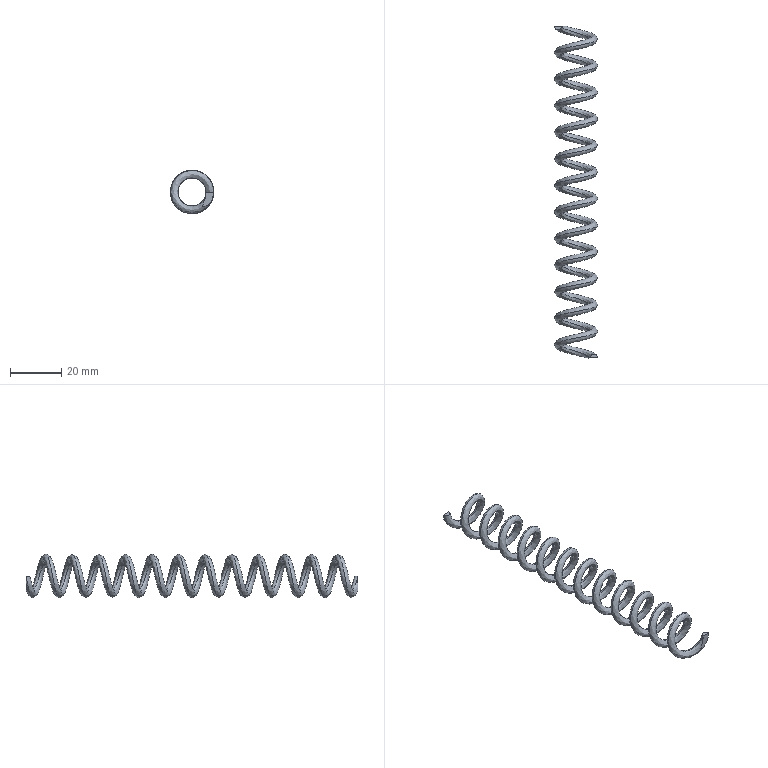Part | SolidWorks | features ICE 1, Sweep 1 | 1 solid | 6 faces | box 17 x 130 x 17 mm | volume 3869 mm3 | plane 4 | spline 2